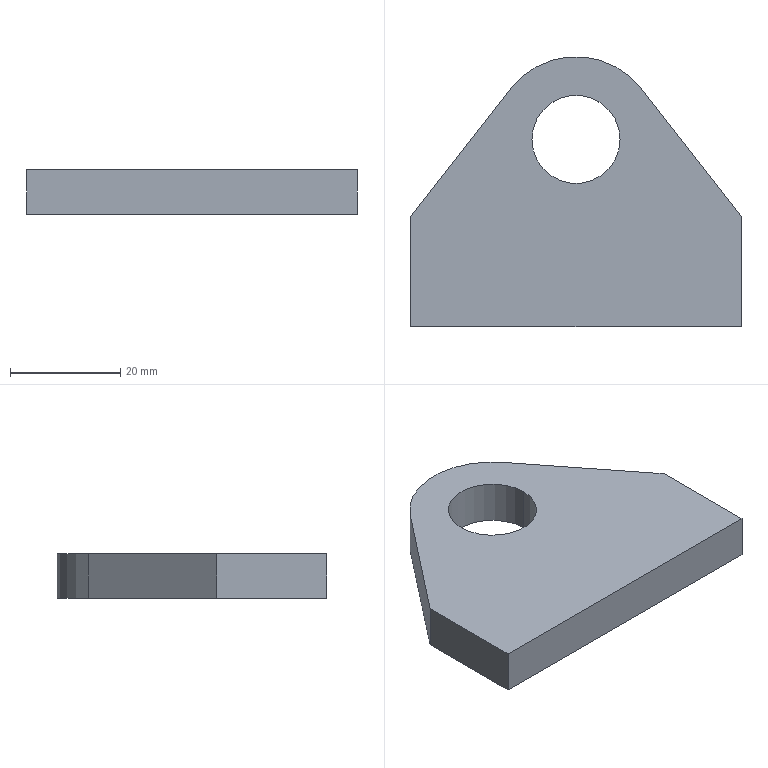Part | SolidWorks | features Extrusion 1 | 1 solid | 10 faces | box 60 x 49 x 8 mm | volume 16525 mm3 | plane 7 | cylinder 3 | commonest cylinder face diameters 16 x2 30 x1
STEP:
#1=CARTESIAN_POINT('',(22.,34.,8.));
#2=VERTEX_POINT('',#1);
#3=CARTESIAN_POINT('',(38.,34.,8.));
#4=VERTEX_POINT('',#3);
#5=CARTESIAN_POINT('',(30.,34.,8.));
#6=DIRECTION('',(0.,0.,1.));
#7=DIRECTION('',(1.,0.,0.));
#8=AXIS2_PLACEMENT_3D('',#5,#6,#7);
#9=CIRCLE('',#8,8.);
#10=EDGE_CURVE('',#2,#4,#9,.T.);
#11=ORIENTED_EDGE('',*,*,#10,.T.);
#12=CARTESIAN_POINT('',(38.,34.,0.));
#13=VERTEX_POINT('',#12);
#14=CARTESIAN_POINT('',(38.,34.,8.));
#15=DIRECTION('',(0.,0.,-1.));
#16=VECTOR('',#15,1000.);
#17=LINE('',#14,#16);
#18=EDGE_CURVE('',#4,#13,#17,.T.);
#19=ORIENTED_EDGE('',*,*,#18,.T.);
#20=CARTESIAN_POINT('',(22.,34.,0.));
#21=VERTEX_POINT('',#20);
#22=CARTESIAN_POINT('',(30.,34.,0.));
#23=DIRECTION('',(0.,0.,1.));
#24=DIRECTION('',(1.,0.,0.));
#25=AXIS2_PLACEMENT_3D('',#22,#23,#24);
#26=CIRCLE('',#25,8.);
#27=EDGE_CURVE('',#21,#13,#26,.T.);
#28=ORIENTED_EDGE('',*,*,#27,.F.);
#29=CARTESIAN_POINT('',(22.,34.,8.));
#30=DIRECTION('',(0.,0.,-1.));
#31=VECTOR('',#30,1000.);
#32=LINE('',#29,#31);
#33=EDGE_CURVE('',#2,#21,#32,.T.);
#34=ORIENTED_EDGE('',*,*,#33,.F.);
#35=EDGE_LOOP('',(#11,#19,#28,#34));
#36=FACE_OUTER_BOUND('',#35,.T.);
#37=CARTESIAN_POINT('',(30.,34.,8.));
#38=DIRECTION('',(0.,0.,-1.));
#39=DIRECTION('',(-1.,0.,0.));
#40=AXIS2_PLACEMENT_3D('',#37,#38,#39);
#41=CYLINDRICAL_SURFACE('',#40,8.);
#42=ADVANCED_FACE('',(#36),#41,.F.);
#43=CARTESIAN_POINT('',(0.,0.,8.));
#44=VERTEX_POINT('',#43);
#45=CARTESIAN_POINT('',(60.,0.,8.));
#46=VERTEX_POINT('',#45);
#47=CARTESIAN_POINT('',(0.,0.,8.));
#48=DIRECTION('',(1.,0.,0.));
#49=VECTOR('',#48,1000.);
#50=LINE('',#47,#49);
#51=EDGE_CURVE('',#44,#46,#50,.T.);
#52=ORIENTED_EDGE('',*,*,#51,.T.);
#53=CARTESIAN_POINT('',(60.,20.,8.));
#54=VERTEX_POINT('',#53);
#55=CARTESIAN_POINT('',(60.,0.,8.));
#56=DIRECTION('',(0.,1.,0.));
#57=VECTOR('',#56,1000.);
#58=LINE('',#55,#57);
#59=EDGE_CURVE('',#46,#54,#58,.T.);
#60=ORIENTED_EDGE('',*,*,#59,.T.);
#61=CARTESIAN_POINT('',(41.814,43.243,8.));
#62=VERTEX_POINT('',#61);
#63=CARTESIAN_POINT('',(60.,20.,8.));
#64=DIRECTION('',(-0.6162,0.7876,0.));
#65=VECTOR('',#64,1000.);
#66=LINE('',#63,#65);
#67=EDGE_CURVE('',#54,#62,#66,.T.);
#68=ORIENTED_EDGE('',*,*,#67,.T.);
#69=CARTESIAN_POINT('',(18.186,43.243,8.));
#70=VERTEX_POINT('',#69);
#71=CARTESIAN_POINT('',(30.,34.,8.));
#72=DIRECTION('',(0.,0.,1.));
#73=DIRECTION('',(1.,0.,0.));
#74=AXIS2_PLACEMENT_3D('',#71,#72,#73);
#75=CIRCLE('',#74,15.);
#76=EDGE_CURVE('',#62,#70,#75,.T.);
#77=ORIENTED_EDGE('',*,*,#76,.T.);
#78=CARTESIAN_POINT('',(0.,20.,8.));
#79=VERTEX_POINT('',#78);
#80=CARTESIAN_POINT('',(0.,20.,8.));
#81=DIRECTION('',(-0.6162,-0.7876,0.));
#82=VECTOR('',#81,1000.);
#83=LINE('',#80,#82);
#84=EDGE_CURVE('',#70,#79,#83,.T.);
#85=ORIENTED_EDGE('',*,*,#84,.T.);
#86=CARTESIAN_POINT('',(0.,0.,8.));
#87=DIRECTION('',(0.,-1.,0.));
#88=VECTOR('',#87,1000.);
#89=LINE('',#86,#88);
#90=EDGE_CURVE('',#79,#44,#89,.T.);
#91=ORIENTED_EDGE('',*,*,#90,.T.);
#92=EDGE_LOOP('',(#52,#60,#68,#77,#85,#91));
#93=FACE_OUTER_BOUND('',#92,.T.);
#94=ORIENTED_EDGE('',*,*,#10,.F.);
#95=CARTESIAN_POINT('',(30.,34.,8.));
#96=DIRECTION('',(0.,0.,1.));
#97=DIRECTION('',(1.,0.,0.));
#98=AXIS2_PLACEMENT_3D('',#95,#96,#97);
#99=CIRCLE('',#98,8.);
#100=EDGE_CURVE('',#4,#2,#99,.T.);
#101=ORIENTED_EDGE('',*,*,#100,.F.);
#102=EDGE_LOOP('',(#94,#101));
#103=FACE_BOUND('',#102,.T.);
#104=CARTESIAN_POINT('',(30.,34.,8.));
#105=DIRECTION('',(0.,0.,1.));
#106=DIRECTION('',(1.,0.,0.));
#107=AXIS2_PLACEMENT_3D('',#104,#105,#106);
#108=PLANE('',#107);
#109=ADVANCED_FACE('',(#93,#103),#108,.T.);
#110=CARTESIAN_POINT('',(0.,0.,0.));
#111=VERTEX_POINT('',#110);
#112=CARTESIAN_POINT('',(60.,0.,0.));
#113=VERTEX_POINT('',#112);
#114=CARTESIAN_POINT('',(0.,0.,0.));
#115=DIRECTION('',(1.,0.,0.));
#116=VECTOR('',#115,1000.);
#117=LINE('',#114,#116);
#118=EDGE_CURVE('',#111,#113,#117,.T.);
#119=ORIENTED_EDGE('',*,*,#118,.F.);
#120=CARTESIAN_POINT('',(0.,20.,0.));
#121=VERTEX_POINT('',#120);
#122=CARTESIAN_POINT('',(0.,0.,0.));
#123=DIRECTION('',(0.,-1.,0.));
#124=VECTOR('',#123,1000.);
#125=LINE('',#122,#124);
#126=EDGE_CURVE('',#121,#111,#125,.T.);
#127=ORIENTED_EDGE('',*,*,#126,.F.);
#128=CARTESIAN_POINT('',(18.186,43.243,0.));
#129=VERTEX_POINT('',#128);
#130=CARTESIAN_POINT('',(0.,20.,0.));
#131=DIRECTION('',(-0.6162,-0.7876,0.));
#132=VECTOR('',#131,1000.);
#133=LINE('',#130,#132);
#134=EDGE_CURVE('',#129,#121,#133,.T.);
#135=ORIENTED_EDGE('',*,*,#134,.F.);
#136=CARTESIAN_POINT('',(41.814,43.243,0.));
#137=VERTEX_POINT('',#136);
#138=CARTESIAN_POINT('',(30.,34.,0.));
#139=DIRECTION('',(0.,0.,1.));
#140=DIRECTION('',(1.,0.,0.));
#141=AXIS2_PLACEMENT_3D('',#138,#139,#140);
#142=CIRCLE('',#141,15.);
#143=EDGE_CURVE('',#137,#129,#142,.T.);
#144=ORIENTED_EDGE('',*,*,#143,.F.);
#145=CARTESIAN_POINT('',(60.,20.,0.));
#146=VERTEX_POINT('',#145);
#147=CARTESIAN_POINT('',(60.,20.,0.));
#148=DIRECTION('',(-0.6162,0.7876,0.));
#149=VECTOR('',#148,1000.);
#150=LINE('',#147,#149);
#151=EDGE_CURVE('',#146,#137,#150,.T.);
#152=ORIENTED_EDGE('',*,*,#151,.F.);
#153=CARTESIAN_POINT('',(60.,0.,0.));
#154=DIRECTION('',(0.,1.,0.));
#155=VECTOR('',#154,1000.);
#156=LINE('',#153,#155);
#157=EDGE_CURVE('',#113,#146,#156,.T.);
#158=ORIENTED_EDGE('',*,*,#157,.F.);
#159=EDGE_LOOP('',(#119,#127,#135,#144,#152,#158));
#160=FACE_OUTER_BOUND('',#159,.T.);
#161=ORIENTED_EDGE('',*,*,#27,.T.);
#162=CARTESIAN_POINT('',(30.,34.,0.));
#163=DIRECTION('',(0.,0.,1.));
#164=DIRECTION('',(1.,0.,0.));
#165=AXIS2_PLACEMENT_3D('',#162,#163,#164);
#166=CIRCLE('',#165,8.);
#167=EDGE_CURVE('',#13,#21,#166,.T.);
#168=ORIENTED_EDGE('',*,*,#167,.T.);
#169=EDGE_LOOP('',(#161,#168));
#170=FACE_BOUND('',#169,.T.);
#171=CARTESIAN_POINT('',(30.,34.,0.));
#172=DIRECTION('',(0.,0.,1.));
#173=DIRECTION('',(1.,0.,0.));
#174=AXIS2_PLACEMENT_3D('',#171,#172,#173);
#175=PLANE('',#174);
#176=ADVANCED_FACE('',(#160,#170),#175,.F.);
#177=ORIENTED_EDGE('',*,*,#118,.T.);
#178=CARTESIAN_POINT('',(60.,0.,8.));
#179=DIRECTION('',(0.,0.,-1.));
#180=VECTOR('',#179,1000.);
#181=LINE('',#178,#180);
#182=EDGE_CURVE('',#46,#113,#181,.T.);
#183=ORIENTED_EDGE('',*,*,#182,.F.);
#184=ORIENTED_EDGE('',*,*,#51,.F.);
#185=CARTESIAN_POINT('',(0.,0.,8.));
#186=DIRECTION('',(0.,0.,-1.));
#187=VECTOR('',#186,1000.);
#188=LINE('',#185,#187);
#189=EDGE_CURVE('',#44,#111,#188,.T.);
#190=ORIENTED_EDGE('',*,*,#189,.T.);
#191=EDGE_LOOP('',(#177,#183,#184,#190));
#192=FACE_OUTER_BOUND('',#191,.T.);
#193=CARTESIAN_POINT('',(0.,0.,8.));
#194=DIRECTION('',(0.,1.,0.));
#195=DIRECTION('',(0.,0.,1.));
#196=AXIS2_PLACEMENT_3D('',#193,#194,#195);
#197=PLANE('',#196);
#198=ADVANCED_FACE('',(#192),#197,.F.);
#199=ORIENTED_EDGE('',*,*,#157,.T.);
#200=CARTESIAN_POINT('',(60.,20.,8.));
#201=DIRECTION('',(0.,0.,-1.));
#202=VECTOR('',#201,1000.);
#203=LINE('',#200,#202);
#204=EDGE_CURVE('',#54,#146,#203,.T.);
#205=ORIENTED_EDGE('',*,*,#204,.F.);
#206=ORIENTED_EDGE('',*,*,#59,.F.);
#207=ORIENTED_EDGE('',*,*,#182,.T.);
#208=EDGE_LOOP('',(#199,#205,#206,#207));
#209=FACE_OUTER_BOUND('',#208,.T.);
#210=CARTESIAN_POINT('',(60.,0.,8.));
#211=DIRECTION('',(-1.,0.,0.));
#212=DIRECTION('',(0.,0.,1.));
#213=AXIS2_PLACEMENT_3D('',#210,#211,#212);
#214=PLANE('',#213);
#215=ADVANCED_FACE('',(#209),#214,.F.);
#216=ORIENTED_EDGE('',*,*,#151,.T.);
#217=CARTESIAN_POINT('',(41.814,43.243,8.));
#218=DIRECTION('',(0.,0.,-1.));
#219=VECTOR('',#218,1000.);
#220=LINE('',#217,#219);
#221=EDGE_CURVE('',#62,#137,#220,.T.);
#222=ORIENTED_EDGE('',*,*,#221,.F.);
#223=ORIENTED_EDGE('',*,*,#67,.F.);
#224=ORIENTED_EDGE('',*,*,#204,.T.);
#225=EDGE_LOOP('',(#216,#222,#223,#224));
#226=FACE_OUTER_BOUND('',#225,.T.);
#227=CARTESIAN_POINT('',(60.,20.,8.));
#228=DIRECTION('',(-0.7876,-0.6162,0.));
#229=DIRECTION('',(0.6162,-0.7876,0.));
#230=AXIS2_PLACEMENT_3D('',#227,#228,#229);
#231=PLANE('',#230);
#232=ADVANCED_FACE('',(#226),#231,.F.);
#233=ORIENTED_EDGE('',*,*,#143,.T.);
#234=CARTESIAN_POINT('',(18.186,43.243,8.));
#235=DIRECTION('',(0.,0.,-1.));
#236=VECTOR('',#235,1000.);
#237=LINE('',#234,#236);
#238=EDGE_CURVE('',#70,#129,#237,.T.);
#239=ORIENTED_EDGE('',*,*,#238,.F.);
#240=ORIENTED_EDGE('',*,*,#76,.F.);
#241=ORIENTED_EDGE('',*,*,#221,.T.);
#242=EDGE_LOOP('',(#233,#239,#240,#241));
#243=FACE_OUTER_BOUND('',#242,.T.);
#244=CARTESIAN_POINT('',(30.,34.,8.));
#245=DIRECTION('',(0.,0.,-1.));
#246=DIRECTION('',(-1.,0.,0.));
#247=AXIS2_PLACEMENT_3D('',#244,#245,#246);
#248=CYLINDRICAL_SURFACE('',#247,15.);
#249=ADVANCED_FACE('',(#243),#248,.T.);
#250=ORIENTED_EDGE('',*,*,#134,.T.);
#251=CARTESIAN_POINT('',(0.,20.,8.));
#252=DIRECTION('',(0.,0.,-1.));
#253=VECTOR('',#252,1000.);
#254=LINE('',#251,#253);
#255=EDGE_CURVE('',#79,#121,#254,.T.);
#256=ORIENTED_EDGE('',*,*,#255,.F.);
#257=ORIENTED_EDGE('',*,*,#84,.F.);
#258=ORIENTED_EDGE('',*,*,#238,.T.);
#259=EDGE_LOOP('',(#250,#256,#257,#258));
#260=FACE_OUTER_BOUND('',#259,.T.);
#261=CARTESIAN_POINT('',(0.,20.,8.));
#262=DIRECTION('',(0.7876,-0.6162,0.));
#263=DIRECTION('',(0.6162,0.7876,0.));
#264=AXIS2_PLACEMENT_3D('',#261,#262,#263);
#265=PLANE('',#264);
#266=ADVANCED_FACE('',(#260),#265,.F.);
#267=ORIENTED_EDGE('',*,*,#126,.T.);
#268=ORIENTED_EDGE('',*,*,#189,.F.);
#269=ORIENTED_EDGE('',*,*,#90,.F.);
#270=ORIENTED_EDGE('',*,*,#255,.T.);
#271=EDGE_LOOP('',(#267,#268,#269,#270));
#272=FACE_OUTER_BOUND('',#271,.T.);
#273=CARTESIAN_POINT('',(0.,0.,8.));
#274=DIRECTION('',(1.,0.,0.));
#275=DIRECTION('',(0.,0.,-1.));
#276=AXIS2_PLACEMENT_3D('',#273,#274,#275);
#277=PLANE('',#276);
#278=ADVANCED_FACE('',(#272),#277,.F.);
#279=ORIENTED_EDGE('',*,*,#18,.F.);
#280=ORIENTED_EDGE('',*,*,#100,.T.);
#281=ORIENTED_EDGE('',*,*,#33,.T.);
#282=ORIENTED_EDGE('',*,*,#167,.F.);
#283=EDGE_LOOP('',(#279,#280,#281,#282));
#284=FACE_OUTER_BOUND('',#283,.T.);
#285=CARTESIAN_POINT('',(30.,34.,8.));
#286=DIRECTION('',(0.,0.,-1.));
#287=DIRECTION('',(-1.,0.,0.));
#288=AXIS2_PLACEMENT_3D('',#285,#286,#287);
#289=CYLINDRICAL_SURFACE('',#288,8.);
#290=ADVANCED_FACE('',(#284),#289,.F.);
#291=CLOSED_SHELL('',(#42,#109,#176,#198,#215,#232,#249,#266,#278,#290));
#292=MANIFOLD_SOLID_BREP('',#291);
#293=CARTESIAN_POINT('',(0.,0.,0.));
#294=DIRECTION('',(0.,0.,1.));
#295=DIRECTION('',(1.,0.,0.));
#296=AXIS2_PLACEMENT_3D('',#293,#294,#295);
#297=(LENGTH_UNIT()NAMED_UNIT(*)SI_UNIT(.MILLI.,.METRE.));
#298=UNCERTAINTY_MEASURE_WITH_UNIT(LENGTH_MEASURE(0.00001),#297,'','');
#299=(NAMED_UNIT(*)PLANE_ANGLE_UNIT()SI_UNIT($,.RADIAN.));
#300=(NAMED_UNIT(*)SI_UNIT($,.STERADIAN.)SOLID_ANGLE_UNIT());
#301=(GEOMETRIC_REPRESENTATION_CONTEXT(3)GLOBAL_UNCERTAINTY_ASSIGNED_CONTEXT((#298))GLOBAL_UNIT_ASSIGNED_CONTEXT((#297,#299,#300))REPRESENTATION_CONTEXT('',''));
#302=ADVANCED_BREP_SHAPE_REPRESENTATION('',(#292,#296),#301);